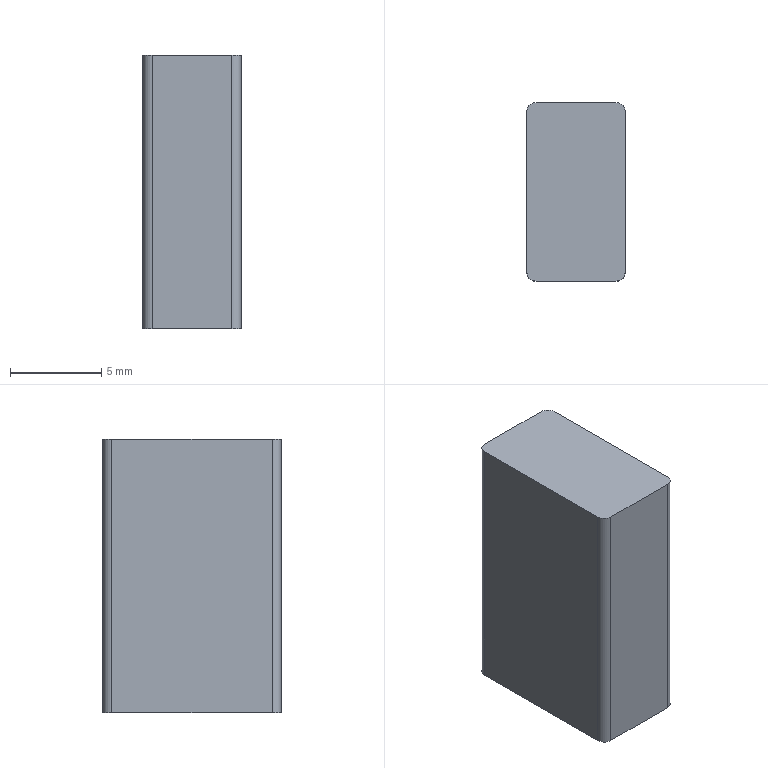Part | NX | features BREP 1 | 1 solid | 10 faces | box 5.385 x 9.783 x 15 mm | volume 786.93 mm3 | plane 6 | cylinder 4 | commonest cylinder face diameters 1 x4
STEP:
#1=CARTESIAN_POINT('',(-2.192,4.891,-25.6));
#2=VERTEX_POINT('',#1);
#3=CARTESIAN_POINT('',(-2.692,4.391,-25.6));
#4=VERTEX_POINT('',#3);
#5=CARTESIAN_POINT('',(-2.192,4.391,-25.6));
#6=DIRECTION('',(0.,0.,1.));
#7=DIRECTION('',(1.,0.,0.));
#8=AXIS2_PLACEMENT_3D('',#5,#6,#7);
#9=CIRCLE('',#8,0.5);
#10=EDGE_CURVE('',#2,#4,#9,.T.);
#11=ORIENTED_EDGE('',*,*,#10,.F.);
#12=CARTESIAN_POINT('',(-2.192,4.891,-40.6));
#13=VERTEX_POINT('',#12);
#14=CARTESIAN_POINT('',(-2.192,4.891,-40.6));
#15=DIRECTION('',(0.,0.,1.));
#16=VECTOR('',#15,1000.);
#17=LINE('',#14,#16);
#18=EDGE_CURVE('',#13,#2,#17,.T.);
#19=ORIENTED_EDGE('',*,*,#18,.F.);
#20=CARTESIAN_POINT('',(-2.692,4.391,-40.6));
#21=VERTEX_POINT('',#20);
#22=CARTESIAN_POINT('',(-2.192,4.391,-40.6));
#23=DIRECTION('',(0.,0.,1.));
#24=DIRECTION('',(1.,0.,0.));
#25=AXIS2_PLACEMENT_3D('',#22,#23,#24);
#26=CIRCLE('',#25,0.5);
#27=EDGE_CURVE('',#13,#21,#26,.T.);
#28=ORIENTED_EDGE('',*,*,#27,.T.);
#29=CARTESIAN_POINT('',(-2.692,4.391,-40.6));
#30=DIRECTION('',(0.,0.,1.));
#31=VECTOR('',#30,1000.);
#32=LINE('',#29,#31);
#33=EDGE_CURVE('',#21,#4,#32,.T.);
#34=ORIENTED_EDGE('',*,*,#33,.T.);
#35=EDGE_LOOP('',(#11,#19,#28,#34));
#36=FACE_BOUND('',#35,.T.);
#37=CARTESIAN_POINT('',(-2.192,4.391,-40.6));
#38=DIRECTION('',(0.,0.,1.));
#39=DIRECTION('',(-1.,0.,0.));
#40=AXIS2_PLACEMENT_3D('',#37,#38,#39);
#41=CYLINDRICAL_SURFACE('',#40,0.5);
#42=ADVANCED_FACE('',(#36),#41,.T.);
#43=CARTESIAN_POINT('',(-2.692,-4.391,-25.6));
#44=VERTEX_POINT('',#43);
#45=CARTESIAN_POINT('',(-2.692,-4.391,-25.6));
#46=DIRECTION('',(0.,1.,0.));
#47=VECTOR('',#46,1000.);
#48=LINE('',#45,#47);
#49=EDGE_CURVE('',#44,#4,#48,.T.);
#50=ORIENTED_EDGE('',*,*,#49,.T.);
#51=ORIENTED_EDGE('',*,*,#33,.F.);
#52=CARTESIAN_POINT('',(-2.692,-4.391,-40.6));
#53=VERTEX_POINT('',#52);
#54=CARTESIAN_POINT('',(-2.692,-4.391,-40.6));
#55=DIRECTION('',(0.,1.,0.));
#56=VECTOR('',#55,1000.);
#57=LINE('',#54,#56);
#58=EDGE_CURVE('',#53,#21,#57,.T.);
#59=ORIENTED_EDGE('',*,*,#58,.F.);
#60=CARTESIAN_POINT('',(-2.692,-4.391,-40.6));
#61=DIRECTION('',(0.,0.,1.));
#62=VECTOR('',#61,1000.);
#63=LINE('',#60,#62);
#64=EDGE_CURVE('',#53,#44,#63,.T.);
#65=ORIENTED_EDGE('',*,*,#64,.T.);
#66=EDGE_LOOP('',(#50,#51,#59,#65));
#67=FACE_BOUND('',#66,.T.);
#68=CARTESIAN_POINT('',(-2.692,-4.391,-40.6));
#69=DIRECTION('',(1.,0.,0.));
#70=DIRECTION('',(0.,-1.,0.));
#71=AXIS2_PLACEMENT_3D('',#68,#69,#70);
#72=PLANE('',#71);
#73=ADVANCED_FACE('',(#67),#72,.F.);
#74=CARTESIAN_POINT('',(-2.192,-4.891,-25.6));
#75=VERTEX_POINT('',#74);
#76=CARTESIAN_POINT('',(-2.192,-4.391,-25.6));
#77=DIRECTION('',(0.,0.,1.));
#78=DIRECTION('',(1.,0.,0.));
#79=AXIS2_PLACEMENT_3D('',#76,#77,#78);
#80=CIRCLE('',#79,0.5);
#81=EDGE_CURVE('',#44,#75,#80,.T.);
#82=ORIENTED_EDGE('',*,*,#81,.F.);
#83=ORIENTED_EDGE('',*,*,#64,.F.);
#84=CARTESIAN_POINT('',(-2.192,-4.891,-40.6));
#85=VERTEX_POINT('',#84);
#86=CARTESIAN_POINT('',(-2.192,-4.391,-40.6));
#87=DIRECTION('',(0.,0.,1.));
#88=DIRECTION('',(1.,0.,0.));
#89=AXIS2_PLACEMENT_3D('',#86,#87,#88);
#90=CIRCLE('',#89,0.5);
#91=EDGE_CURVE('',#53,#85,#90,.T.);
#92=ORIENTED_EDGE('',*,*,#91,.T.);
#93=CARTESIAN_POINT('',(-2.192,-4.891,-40.6));
#94=DIRECTION('',(0.,0.,1.));
#95=VECTOR('',#94,1000.);
#96=LINE('',#93,#95);
#97=EDGE_CURVE('',#85,#75,#96,.T.);
#98=ORIENTED_EDGE('',*,*,#97,.T.);
#99=EDGE_LOOP('',(#82,#83,#92,#98));
#100=FACE_BOUND('',#99,.T.);
#101=CARTESIAN_POINT('',(-2.192,-4.391,-40.6));
#102=DIRECTION('',(0.,0.,1.));
#103=DIRECTION('',(-1.,0.,0.));
#104=AXIS2_PLACEMENT_3D('',#101,#102,#103);
#105=CYLINDRICAL_SURFACE('',#104,0.5);
#106=ADVANCED_FACE('',(#100),#105,.T.);
#107=CARTESIAN_POINT('',(2.192,-4.891,-25.6));
#108=VERTEX_POINT('',#107);
#109=CARTESIAN_POINT('',(2.192,-4.891,-25.6));
#110=DIRECTION('',(-1.,0.,0.));
#111=VECTOR('',#110,1000.);
#112=LINE('',#109,#111);
#113=EDGE_CURVE('',#108,#75,#112,.T.);
#114=ORIENTED_EDGE('',*,*,#113,.T.);
#115=ORIENTED_EDGE('',*,*,#97,.F.);
#116=CARTESIAN_POINT('',(2.192,-4.891,-40.6));
#117=VERTEX_POINT('',#116);
#118=CARTESIAN_POINT('',(2.192,-4.891,-40.6));
#119=DIRECTION('',(-1.,0.,0.));
#120=VECTOR('',#119,1000.);
#121=LINE('',#118,#120);
#122=EDGE_CURVE('',#117,#85,#121,.T.);
#123=ORIENTED_EDGE('',*,*,#122,.F.);
#124=CARTESIAN_POINT('',(2.192,-4.891,-40.6));
#125=DIRECTION('',(0.,0.,1.));
#126=VECTOR('',#125,1000.);
#127=LINE('',#124,#126);
#128=EDGE_CURVE('',#117,#108,#127,.T.);
#129=ORIENTED_EDGE('',*,*,#128,.T.);
#130=EDGE_LOOP('',(#114,#115,#123,#129));
#131=FACE_BOUND('',#130,.T.);
#132=CARTESIAN_POINT('',(2.192,-4.891,-40.6));
#133=DIRECTION('',(0.,1.,0.));
#134=DIRECTION('',(0.,0.,-1.));
#135=AXIS2_PLACEMENT_3D('',#132,#133,#134);
#136=PLANE('',#135);
#137=ADVANCED_FACE('',(#131),#136,.F.);
#138=CARTESIAN_POINT('',(2.692,-4.391,-25.6));
#139=VERTEX_POINT('',#138);
#140=CARTESIAN_POINT('',(2.192,-4.391,-25.6));
#141=DIRECTION('',(0.,0.,1.));
#142=DIRECTION('',(1.,0.,0.));
#143=AXIS2_PLACEMENT_3D('',#140,#141,#142);
#144=CIRCLE('',#143,0.5);
#145=EDGE_CURVE('',#108,#139,#144,.T.);
#146=ORIENTED_EDGE('',*,*,#145,.F.);
#147=ORIENTED_EDGE('',*,*,#128,.F.);
#148=CARTESIAN_POINT('',(2.692,-4.391,-40.6));
#149=VERTEX_POINT('',#148);
#150=CARTESIAN_POINT('',(2.192,-4.391,-40.6));
#151=DIRECTION('',(0.,0.,1.));
#152=DIRECTION('',(1.,0.,0.));
#153=AXIS2_PLACEMENT_3D('',#150,#151,#152);
#154=CIRCLE('',#153,0.5);
#155=EDGE_CURVE('',#117,#149,#154,.T.);
#156=ORIENTED_EDGE('',*,*,#155,.T.);
#157=CARTESIAN_POINT('',(2.692,-4.391,-40.6));
#158=DIRECTION('',(0.,0.,1.));
#159=VECTOR('',#158,1000.);
#160=LINE('',#157,#159);
#161=EDGE_CURVE('',#149,#139,#160,.T.);
#162=ORIENTED_EDGE('',*,*,#161,.T.);
#163=EDGE_LOOP('',(#146,#147,#156,#162));
#164=FACE_BOUND('',#163,.T.);
#165=CARTESIAN_POINT('',(2.192,-4.391,-40.6));
#166=DIRECTION('',(0.,0.,1.));
#167=DIRECTION('',(-1.,0.,0.));
#168=AXIS2_PLACEMENT_3D('',#165,#166,#167);
#169=CYLINDRICAL_SURFACE('',#168,0.5);
#170=ADVANCED_FACE('',(#164),#169,.T.);
#171=CARTESIAN_POINT('',(2.692,4.391,-25.6));
#172=VERTEX_POINT('',#171);
#173=CARTESIAN_POINT('',(2.692,4.391,-25.6));
#174=DIRECTION('',(0.,-1.,0.));
#175=VECTOR('',#174,1000.);
#176=LINE('',#173,#175);
#177=EDGE_CURVE('',#172,#139,#176,.T.);
#178=ORIENTED_EDGE('',*,*,#177,.T.);
#179=ORIENTED_EDGE('',*,*,#161,.F.);
#180=CARTESIAN_POINT('',(2.692,4.391,-40.6));
#181=VERTEX_POINT('',#180);
#182=CARTESIAN_POINT('',(2.692,4.391,-40.6));
#183=DIRECTION('',(0.,-1.,0.));
#184=VECTOR('',#183,1000.);
#185=LINE('',#182,#184);
#186=EDGE_CURVE('',#181,#149,#185,.T.);
#187=ORIENTED_EDGE('',*,*,#186,.F.);
#188=CARTESIAN_POINT('',(2.692,4.391,-40.6));
#189=DIRECTION('',(0.,0.,1.));
#190=VECTOR('',#189,1000.);
#191=LINE('',#188,#190);
#192=EDGE_CURVE('',#181,#172,#191,.T.);
#193=ORIENTED_EDGE('',*,*,#192,.T.);
#194=EDGE_LOOP('',(#178,#179,#187,#193));
#195=FACE_BOUND('',#194,.T.);
#196=CARTESIAN_POINT('',(2.692,4.391,-40.6));
#197=DIRECTION('',(-1.,0.,0.));
#198=DIRECTION('',(0.,1.,0.));
#199=AXIS2_PLACEMENT_3D('',#196,#197,#198);
#200=PLANE('',#199);
#201=ADVANCED_FACE('',(#195),#200,.F.);
#202=CARTESIAN_POINT('',(2.192,4.891,-25.6));
#203=VERTEX_POINT('',#202);
#204=CARTESIAN_POINT('',(2.192,4.391,-25.6));
#205=DIRECTION('',(0.,0.,1.));
#206=DIRECTION('',(1.,0.,0.));
#207=AXIS2_PLACEMENT_3D('',#204,#205,#206);
#208=CIRCLE('',#207,0.5);
#209=EDGE_CURVE('',#172,#203,#208,.T.);
#210=ORIENTED_EDGE('',*,*,#209,.F.);
#211=ORIENTED_EDGE('',*,*,#192,.F.);
#212=CARTESIAN_POINT('',(2.192,4.891,-40.6));
#213=VERTEX_POINT('',#212);
#214=CARTESIAN_POINT('',(2.192,4.391,-40.6));
#215=DIRECTION('',(0.,0.,1.));
#216=DIRECTION('',(1.,0.,0.));
#217=AXIS2_PLACEMENT_3D('',#214,#215,#216);
#218=CIRCLE('',#217,0.5);
#219=EDGE_CURVE('',#181,#213,#218,.T.);
#220=ORIENTED_EDGE('',*,*,#219,.T.);
#221=CARTESIAN_POINT('',(2.192,4.891,-40.6));
#222=DIRECTION('',(0.,0.,1.));
#223=VECTOR('',#222,1000.);
#224=LINE('',#221,#223);
#225=EDGE_CURVE('',#213,#203,#224,.T.);
#226=ORIENTED_EDGE('',*,*,#225,.T.);
#227=EDGE_LOOP('',(#210,#211,#220,#226));
#228=FACE_BOUND('',#227,.T.);
#229=CARTESIAN_POINT('',(2.192,4.391,-40.6));
#230=DIRECTION('',(0.,0.,1.));
#231=DIRECTION('',(-1.,0.,0.));
#232=AXIS2_PLACEMENT_3D('',#229,#230,#231);
#233=CYLINDRICAL_SURFACE('',#232,0.5);
#234=ADVANCED_FACE('',(#228),#233,.T.);
#235=CARTESIAN_POINT('',(-2.192,4.891,-25.6));
#236=DIRECTION('',(1.,0.,0.));
#237=VECTOR('',#236,1000.);
#238=LINE('',#235,#237);
#239=EDGE_CURVE('',#2,#203,#238,.T.);
#240=ORIENTED_EDGE('',*,*,#239,.T.);
#241=ORIENTED_EDGE('',*,*,#225,.F.);
#242=CARTESIAN_POINT('',(-2.192,4.891,-40.6));
#243=DIRECTION('',(1.,0.,0.));
#244=VECTOR('',#243,1000.);
#245=LINE('',#242,#244);
#246=EDGE_CURVE('',#13,#213,#245,.T.);
#247=ORIENTED_EDGE('',*,*,#246,.F.);
#248=ORIENTED_EDGE('',*,*,#18,.T.);
#249=EDGE_LOOP('',(#240,#241,#247,#248));
#250=FACE_BOUND('',#249,.T.);
#251=CARTESIAN_POINT('',(-2.192,4.891,-40.6));
#252=DIRECTION('',(0.,-1.,0.));
#253=DIRECTION('',(0.,0.,1.));
#254=AXIS2_PLACEMENT_3D('',#251,#252,#253);
#255=PLANE('',#254);
#256=ADVANCED_FACE('',(#250),#255,.F.);
#257=ORIENTED_EDGE('',*,*,#27,.F.);
#258=ORIENTED_EDGE('',*,*,#246,.T.);
#259=ORIENTED_EDGE('',*,*,#219,.F.);
#260=ORIENTED_EDGE('',*,*,#186,.T.);
#261=ORIENTED_EDGE('',*,*,#155,.F.);
#262=ORIENTED_EDGE('',*,*,#122,.T.);
#263=ORIENTED_EDGE('',*,*,#91,.F.);
#264=ORIENTED_EDGE('',*,*,#58,.T.);
#265=EDGE_LOOP('',(#257,#258,#259,#260,#261,#262,#263,#264));
#266=FACE_BOUND('',#265,.T.);
#267=CARTESIAN_POINT('',(-2.192,4.391,-40.6));
#268=DIRECTION('',(0.,0.,1.));
#269=DIRECTION('',(-1.,0.,0.));
#270=AXIS2_PLACEMENT_3D('',#267,#268,#269);
#271=PLANE('',#270);
#272=ADVANCED_FACE('',(#266),#271,.F.);
#273=ORIENTED_EDGE('',*,*,#10,.T.);
#274=ORIENTED_EDGE('',*,*,#49,.F.);
#275=ORIENTED_EDGE('',*,*,#81,.T.);
#276=ORIENTED_EDGE('',*,*,#113,.F.);
#277=ORIENTED_EDGE('',*,*,#145,.T.);
#278=ORIENTED_EDGE('',*,*,#177,.F.);
#279=ORIENTED_EDGE('',*,*,#209,.T.);
#280=ORIENTED_EDGE('',*,*,#239,.F.);
#281=EDGE_LOOP('',(#273,#274,#275,#276,#277,#278,#279,#280));
#282=FACE_BOUND('',#281,.T.);
#283=CARTESIAN_POINT('',(-2.192,4.391,-25.6));
#284=DIRECTION('',(0.,0.,1.));
#285=DIRECTION('',(-1.,0.,0.));
#286=AXIS2_PLACEMENT_3D('',#283,#284,#285);
#287=PLANE('',#286);
#288=ADVANCED_FACE('',(#282),#287,.T.);
#289=CLOSED_SHELL('',(#42,#73,#106,#137,#170,#201,#234,#256,#272,#288));
#290=MANIFOLD_SOLID_BREP('',#289);
#291=(LENGTH_UNIT()NAMED_UNIT(*)SI_UNIT(.MILLI.,.METRE.));
#292=UNCERTAINTY_MEASURE_WITH_UNIT(LENGTH_MEASURE(0.00001),#291,'','');
#293=(NAMED_UNIT(*)PLANE_ANGLE_UNIT()SI_UNIT($,.RADIAN.));
#294=(NAMED_UNIT(*)SI_UNIT($,.STERADIAN.)SOLID_ANGLE_UNIT());
#295=(GEOMETRIC_REPRESENTATION_CONTEXT(3)GLOBAL_UNCERTAINTY_ASSIGNED_CONTEXT((#292))GLOBAL_UNIT_ASSIGNED_CONTEXT((#291,#293,#294))REPRESENTATION_CONTEXT('',''));
#296=ADVANCED_BREP_SHAPE_REPRESENTATION('',(#290),#295);